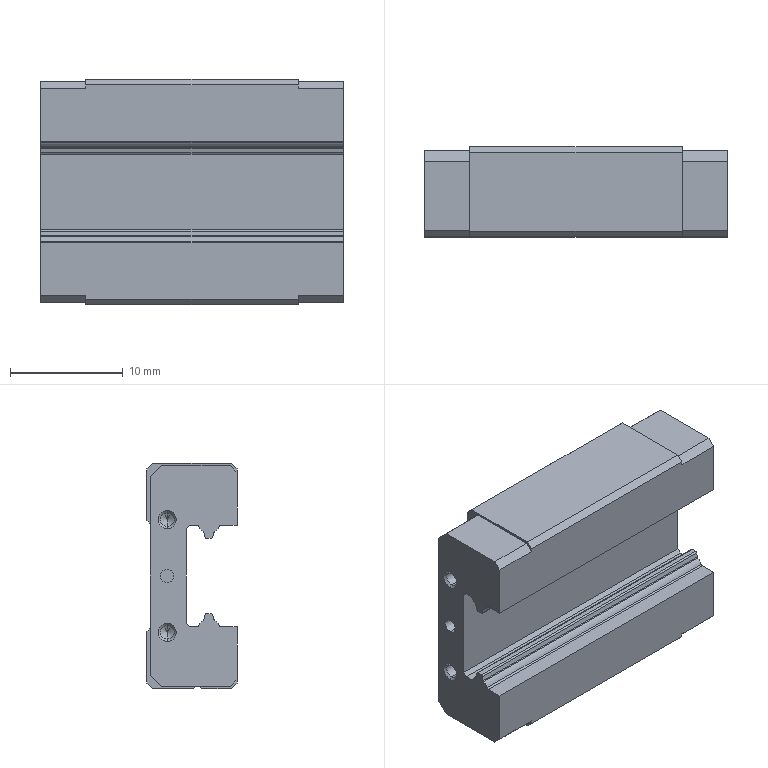Part | STEP file | MGN9CZ0HM | 1 solid | 119 faces | box 26.9 x 8 x 20 mm | volume 3027 mm3 | plane 49 | cylinder 38 | cone 32 | commonest cylinder face diameters 0.3 x12 1.221 x8 2.459 x8 1.2 x4 2 x4 0.8 x2